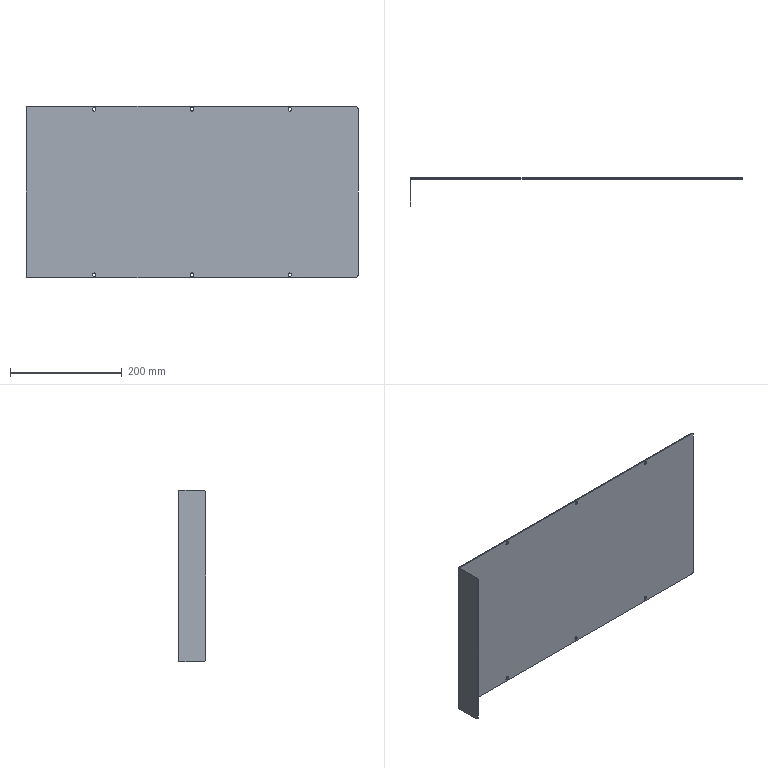Part | SolidWorks | features ICE 2, BreakCorner 1, EdgeFlange 1, Fillet 1, FlatPattern 1, SMBaseFlange 1, SheetMetal 1 | 1 solid | 48 faces | box 595 x 50 x 308 mm | volume 296830 mm3 | cylinder 24 | plane 24 | commonest cylinder face diameters 5 x18 10 x4 0.2 x1 3.2 x1
STEP:
#1=CARTESIAN_POINT('',(-175.,-1.5,-145.));
#2=VERTEX_POINT('',#1);
#3=CARTESIAN_POINT('',(-172.5,-1.5,-147.5));
#4=VERTEX_POINT('',#3);
#5=CARTESIAN_POINT('',(-175.,-1.5,-147.5));
#6=DIRECTION('',(0.,1.,0.));
#7=DIRECTION('',(0.,0.,1.));
#8=AXIS2_PLACEMENT_3D('',#5,#6,#7);
#9=CIRCLE('',#8,2.5);
#10=EDGE_CURVE('',#2,#4,#9,.T.);
#11=ORIENTED_EDGE('',*,*,#10,.F.);
#12=CARTESIAN_POINT('',(-175.,0.,-145.));
#13=VERTEX_POINT('',#12);
#14=CARTESIAN_POINT('',(-175.,-10.,-145.));
#15=DIRECTION('',(0.,1.,0.));
#16=VECTOR('',#15,1000.);
#17=LINE('',#14,#16);
#18=EDGE_CURVE('',#2,#13,#17,.T.);
#19=ORIENTED_EDGE('',*,*,#18,.T.);
#20=CARTESIAN_POINT('',(-172.5,0.,-147.5));
#21=VERTEX_POINT('',#20);
#22=CARTESIAN_POINT('',(-175.,0.,-147.5));
#23=DIRECTION('',(0.,1.,0.));
#24=DIRECTION('',(0.,0.,-1.));
#25=AXIS2_PLACEMENT_3D('',#22,#23,#24);
#26=CIRCLE('',#25,2.5);
#27=EDGE_CURVE('',#13,#21,#26,.T.);
#28=ORIENTED_EDGE('',*,*,#27,.T.);
#29=CARTESIAN_POINT('',(-172.5,-10.,-147.5));
#30=DIRECTION('',(0.,1.,0.));
#31=VECTOR('',#30,1000.);
#32=LINE('',#29,#31);
#33=EDGE_CURVE('',#4,#21,#32,.T.);
#34=ORIENTED_EDGE('',*,*,#33,.F.);
#35=EDGE_LOOP('',(#11,#19,#28,#34));
#36=FACE_OUTER_BOUND('',#35,.T.);
#37=CARTESIAN_POINT('',(-175.,-10.,-147.5));
#38=DIRECTION('',(0.,1.,0.));
#39=DIRECTION('',(0.,0.,1.));
#40=AXIS2_PLACEMENT_3D('',#37,#38,#39);
#41=CYLINDRICAL_SURFACE('',#40,2.5);
#42=ADVANCED_FACE('',(#36),#41,.F.);
#43=CARTESIAN_POINT('',(0.,-1.5,-145.));
#44=VERTEX_POINT('',#43);
#45=CARTESIAN_POINT('',(2.5,-1.5,-147.5));
#46=VERTEX_POINT('',#45);
#47=CARTESIAN_POINT('',(0.,-1.5,-147.5));
#48=DIRECTION('',(0.,1.,0.));
#49=DIRECTION('',(0.,0.,1.));
#50=AXIS2_PLACEMENT_3D('',#47,#48,#49);
#51=CIRCLE('',#50,2.5);
#52=EDGE_CURVE('',#44,#46,#51,.T.);
#53=ORIENTED_EDGE('',*,*,#52,.F.);
#54=CARTESIAN_POINT('',(0.,0.,-145.));
#55=VERTEX_POINT('',#54);
#56=CARTESIAN_POINT('',(0.,-10.,-145.));
#57=DIRECTION('',(0.,1.,0.));
#58=VECTOR('',#57,1000.);
#59=LINE('',#56,#58);
#60=EDGE_CURVE('',#44,#55,#59,.T.);
#61=ORIENTED_EDGE('',*,*,#60,.T.);
#62=CARTESIAN_POINT('',(2.5,0.,-147.5));
#63=VERTEX_POINT('',#62);
#64=CARTESIAN_POINT('',(0.,0.,-147.5));
#65=DIRECTION('',(0.,1.,0.));
#66=DIRECTION('',(0.,0.,-1.));
#67=AXIS2_PLACEMENT_3D('',#64,#65,#66);
#68=CIRCLE('',#67,2.5);
#69=EDGE_CURVE('',#55,#63,#68,.T.);
#70=ORIENTED_EDGE('',*,*,#69,.T.);
#71=CARTESIAN_POINT('',(2.5,-10.,-147.5));
#72=DIRECTION('',(0.,1.,0.));
#73=VECTOR('',#72,1000.);
#74=LINE('',#71,#73);
#75=EDGE_CURVE('',#46,#63,#74,.T.);
#76=ORIENTED_EDGE('',*,*,#75,.F.);
#77=EDGE_LOOP('',(#53,#61,#70,#76));
#78=FACE_OUTER_BOUND('',#77,.T.);
#79=CARTESIAN_POINT('',(0.,-10.,-147.5));
#80=DIRECTION('',(0.,1.,0.));
#81=DIRECTION('',(0.,0.,1.));
#82=AXIS2_PLACEMENT_3D('',#79,#80,#81);
#83=CYLINDRICAL_SURFACE('',#82,2.5);
#84=ADVANCED_FACE('',(#78),#83,.F.);
#85=CARTESIAN_POINT('',(175.,-1.5,-145.));
#86=VERTEX_POINT('',#85);
#87=CARTESIAN_POINT('',(177.5,-1.5,-147.5));
#88=VERTEX_POINT('',#87);
#89=CARTESIAN_POINT('',(175.,-1.5,-147.5));
#90=DIRECTION('',(0.,1.,0.));
#91=DIRECTION('',(0.,0.,1.));
#92=AXIS2_PLACEMENT_3D('',#89,#90,#91);
#93=CIRCLE('',#92,2.5);
#94=EDGE_CURVE('',#86,#88,#93,.T.);
#95=ORIENTED_EDGE('',*,*,#94,.F.);
#96=CARTESIAN_POINT('',(175.,0.,-145.));
#97=VERTEX_POINT('',#96);
#98=CARTESIAN_POINT('',(175.,-10.,-145.));
#99=DIRECTION('',(0.,1.,0.));
#100=VECTOR('',#99,1000.);
#101=LINE('',#98,#100);
#102=EDGE_CURVE('',#86,#97,#101,.T.);
#103=ORIENTED_EDGE('',*,*,#102,.T.);
#104=CARTESIAN_POINT('',(177.5,0.,-147.5));
#105=VERTEX_POINT('',#104);
#106=CARTESIAN_POINT('',(175.,0.,-147.5));
#107=DIRECTION('',(0.,1.,0.));
#108=DIRECTION('',(0.,0.,-1.));
#109=AXIS2_PLACEMENT_3D('',#106,#107,#108);
#110=CIRCLE('',#109,2.5);
#111=EDGE_CURVE('',#97,#105,#110,.T.);
#112=ORIENTED_EDGE('',*,*,#111,.T.);
#113=CARTESIAN_POINT('',(177.5,-10.,-147.5));
#114=DIRECTION('',(0.,1.,0.));
#115=VECTOR('',#114,1000.);
#116=LINE('',#113,#115);
#117=EDGE_CURVE('',#88,#105,#116,.T.);
#118=ORIENTED_EDGE('',*,*,#117,.F.);
#119=EDGE_LOOP('',(#95,#103,#112,#118));
#120=FACE_OUTER_BOUND('',#119,.T.);
#121=CARTESIAN_POINT('',(175.,-10.,-147.5));
#122=DIRECTION('',(0.,1.,0.));
#123=DIRECTION('',(0.,0.,1.));
#124=AXIS2_PLACEMENT_3D('',#121,#122,#123);
#125=CYLINDRICAL_SURFACE('',#124,2.5);
#126=ADVANCED_FACE('',(#120),#125,.F.);
#127=CARTESIAN_POINT('',(175.,-1.5,152.));
#128=VERTEX_POINT('',#127);
#129=CARTESIAN_POINT('',(177.5,-1.5,149.5));
#130=VERTEX_POINT('',#129);
#131=CARTESIAN_POINT('',(175.,-1.5,149.5));
#132=DIRECTION('',(0.,1.,0.));
#133=DIRECTION('',(0.,0.,1.));
#134=AXIS2_PLACEMENT_3D('',#131,#132,#133);
#135=CIRCLE('',#134,2.5);
#136=EDGE_CURVE('',#128,#130,#135,.T.);
#137=ORIENTED_EDGE('',*,*,#136,.F.);
#138=CARTESIAN_POINT('',(175.,0.,152.));
#139=VERTEX_POINT('',#138);
#140=CARTESIAN_POINT('',(175.,-10.,152.));
#141=DIRECTION('',(0.,1.,0.));
#142=VECTOR('',#141,1000.);
#143=LINE('',#140,#142);
#144=EDGE_CURVE('',#128,#139,#143,.T.);
#145=ORIENTED_EDGE('',*,*,#144,.T.);
#146=CARTESIAN_POINT('',(177.5,0.,149.5));
#147=VERTEX_POINT('',#146);
#148=CARTESIAN_POINT('',(175.,0.,149.5));
#149=DIRECTION('',(0.,1.,0.));
#150=DIRECTION('',(0.,0.,1.));
#151=AXIS2_PLACEMENT_3D('',#148,#149,#150);
#152=CIRCLE('',#151,2.5);
#153=EDGE_CURVE('',#139,#147,#152,.T.);
#154=ORIENTED_EDGE('',*,*,#153,.T.);
#155=CARTESIAN_POINT('',(177.5,-10.,149.5));
#156=DIRECTION('',(0.,1.,0.));
#157=VECTOR('',#156,1000.);
#158=LINE('',#155,#157);
#159=EDGE_CURVE('',#130,#147,#158,.T.);
#160=ORIENTED_EDGE('',*,*,#159,.F.);
#161=EDGE_LOOP('',(#137,#145,#154,#160));
#162=FACE_OUTER_BOUND('',#161,.T.);
#163=CARTESIAN_POINT('',(175.,-10.,149.5));
#164=DIRECTION('',(0.,1.,0.));
#165=DIRECTION('',(0.,0.,1.));
#166=AXIS2_PLACEMENT_3D('',#163,#164,#165);
#167=CYLINDRICAL_SURFACE('',#166,2.5);
#168=ADVANCED_FACE('',(#162),#167,.F.);
#169=CARTESIAN_POINT('',(0.,-1.5,152.));
#170=VERTEX_POINT('',#169);
#171=CARTESIAN_POINT('',(2.5,-1.5,149.5));
#172=VERTEX_POINT('',#171);
#173=CARTESIAN_POINT('',(0.,-1.5,149.5));
#174=DIRECTION('',(0.,1.,0.));
#175=DIRECTION('',(0.,0.,1.));
#176=AXIS2_PLACEMENT_3D('',#173,#174,#175);
#177=CIRCLE('',#176,2.5);
#178=EDGE_CURVE('',#170,#172,#177,.T.);
#179=ORIENTED_EDGE('',*,*,#178,.F.);
#180=CARTESIAN_POINT('',(0.,0.,152.));
#181=VERTEX_POINT('',#180);
#182=CARTESIAN_POINT('',(0.,-10.,152.));
#183=DIRECTION('',(0.,1.,0.));
#184=VECTOR('',#183,1000.);
#185=LINE('',#182,#184);
#186=EDGE_CURVE('',#170,#181,#185,.T.);
#187=ORIENTED_EDGE('',*,*,#186,.T.);
#188=CARTESIAN_POINT('',(2.5,0.,149.5));
#189=VERTEX_POINT('',#188);
#190=CARTESIAN_POINT('',(0.,0.,149.5));
#191=DIRECTION('',(0.,1.,0.));
#192=DIRECTION('',(0.,0.,1.));
#193=AXIS2_PLACEMENT_3D('',#190,#191,#192);
#194=CIRCLE('',#193,2.5);
#195=EDGE_CURVE('',#181,#189,#194,.T.);
#196=ORIENTED_EDGE('',*,*,#195,.T.);
#197=CARTESIAN_POINT('',(2.5,-10.,149.5));
#198=DIRECTION('',(0.,1.,0.));
#199=VECTOR('',#198,1000.);
#200=LINE('',#197,#199);
#201=EDGE_CURVE('',#172,#189,#200,.T.);
#202=ORIENTED_EDGE('',*,*,#201,.F.);
#203=EDGE_LOOP('',(#179,#187,#196,#202));
#204=FACE_OUTER_BOUND('',#203,.T.);
#205=CARTESIAN_POINT('',(0.,-10.,149.5));
#206=DIRECTION('',(0.,1.,0.));
#207=DIRECTION('',(0.,0.,1.));
#208=AXIS2_PLACEMENT_3D('',#205,#206,#207);
#209=CYLINDRICAL_SURFACE('',#208,2.5);
#210=ADVANCED_FACE('',(#204),#209,.F.);
#211=CARTESIAN_POINT('',(-175.,-1.5,152.));
#212=VERTEX_POINT('',#211);
#213=CARTESIAN_POINT('',(-172.5,-1.5,149.5));
#214=VERTEX_POINT('',#213);
#215=CARTESIAN_POINT('',(-175.,-1.5,149.5));
#216=DIRECTION('',(0.,1.,0.));
#217=DIRECTION('',(0.,0.,1.));
#218=AXIS2_PLACEMENT_3D('',#215,#216,#217);
#219=CIRCLE('',#218,2.5);
#220=EDGE_CURVE('',#212,#214,#219,.T.);
#221=ORIENTED_EDGE('',*,*,#220,.F.);
#222=CARTESIAN_POINT('',(-175.,0.,152.));
#223=VERTEX_POINT('',#222);
#224=CARTESIAN_POINT('',(-175.,-10.,152.));
#225=DIRECTION('',(0.,1.,0.));
#226=VECTOR('',#225,1000.);
#227=LINE('',#224,#226);
#228=EDGE_CURVE('',#212,#223,#227,.T.);
#229=ORIENTED_EDGE('',*,*,#228,.T.);
#230=CARTESIAN_POINT('',(-172.5,0.,149.5));
#231=VERTEX_POINT('',#230);
#232=CARTESIAN_POINT('',(-175.,0.,149.5));
#233=DIRECTION('',(0.,1.,0.));
#234=DIRECTION('',(0.,0.,1.));
#235=AXIS2_PLACEMENT_3D('',#232,#233,#234);
#236=CIRCLE('',#235,2.5);
#237=EDGE_CURVE('',#223,#231,#236,.T.);
#238=ORIENTED_EDGE('',*,*,#237,.T.);
#239=CARTESIAN_POINT('',(-172.5,-10.,149.5));
#240=DIRECTION('',(0.,1.,0.));
#241=VECTOR('',#240,1000.);
#242=LINE('',#239,#241);
#243=EDGE_CURVE('',#214,#231,#242,.T.);
#244=ORIENTED_EDGE('',*,*,#243,.F.);
#245=EDGE_LOOP('',(#221,#229,#238,#244));
#246=FACE_OUTER_BOUND('',#245,.T.);
#247=CARTESIAN_POINT('',(-175.,-10.,149.5));
#248=DIRECTION('',(0.,1.,0.));
#249=DIRECTION('',(0.,0.,1.));
#250=AXIS2_PLACEMENT_3D('',#247,#248,#249);
#251=CYLINDRICAL_SURFACE('',#250,2.5);
#252=ADVANCED_FACE('',(#246),#251,.F.);
#253=CARTESIAN_POINT('',(292.5,0.,-154.));
#254=VERTEX_POINT('',#253);
#255=CARTESIAN_POINT('',(-295.9,0.,-154.));
#256=VERTEX_POINT('',#255);
#257=CARTESIAN_POINT('',(297.5,0.,-154.));
#258=DIRECTION('',(-1.,0.,0.));
#259=VECTOR('',#258,1000.);
#260=LINE('',#257,#259);
#261=EDGE_CURVE('',#254,#256,#260,.T.);
#262=ORIENTED_EDGE('',*,*,#261,.F.);
#263=CARTESIAN_POINT('',(292.5,-1.5,-154.));
#264=VERTEX_POINT('',#263);
#265=CARTESIAN_POINT('',(292.5,-1.5,-154.));
#266=DIRECTION('',(0.,-1.,0.));
#267=VECTOR('',#266,1000.);
#268=LINE('',#265,#267);
#269=EDGE_CURVE('',#254,#264,#268,.T.);
#270=ORIENTED_EDGE('',*,*,#269,.T.);
#271=CARTESIAN_POINT('',(-295.9,-1.5,-154.));
#272=VERTEX_POINT('',#271);
#273=CARTESIAN_POINT('',(297.5,-1.5,-154.));
#274=DIRECTION('',(-1.,0.,0.));
#275=VECTOR('',#274,1000.);
#276=LINE('',#273,#275);
#277=EDGE_CURVE('',#264,#272,#276,.T.);
#278=ORIENTED_EDGE('',*,*,#277,.T.);
#279=CARTESIAN_POINT('',(-295.9,-1.5,-154.));
#280=DIRECTION('',(0.,1.,0.));
#281=VECTOR('',#280,1000.);
#282=LINE('',#279,#281);
#283=EDGE_CURVE('',#272,#256,#282,.T.);
#284=ORIENTED_EDGE('',*,*,#283,.T.);
#285=EDGE_LOOP('',(#262,#270,#278,#284));
#286=FACE_OUTER_BOUND('',#285,.T.);
#287=CARTESIAN_POINT('',(297.5,-1.5,-154.));
#288=DIRECTION('',(0.,0.,-1.));
#289=DIRECTION('',(-1.,0.,0.));
#290=AXIS2_PLACEMENT_3D('',#287,#288,#289);
#291=PLANE('',#290);
#292=ADVANCED_FACE('',(#286),#291,.T.);
#293=CARTESIAN_POINT('',(-172.5,-1.5,-149.5));
#294=VERTEX_POINT('',#293);
#295=CARTESIAN_POINT('',(-172.5,-1.5,0.));
#296=DIRECTION('',(0.,0.,-1.));
#297=VECTOR('',#296,1000.);
#298=LINE('',#295,#297);
#299=EDGE_CURVE('',#4,#294,#298,.T.);
#300=ORIENTED_EDGE('',*,*,#299,.T.);
#301=CARTESIAN_POINT('',(-177.5,-1.5,-149.5));
#302=VERTEX_POINT('',#301);
#303=CARTESIAN_POINT('',(-175.,-1.5,-149.5));
#304=DIRECTION('',(0.,1.,0.));
#305=DIRECTION('',(0.,0.,1.));
#306=AXIS2_PLACEMENT_3D('',#303,#304,#305);
#307=CIRCLE('',#306,2.5);
#308=EDGE_CURVE('',#294,#302,#307,.T.);
#309=ORIENTED_EDGE('',*,*,#308,.T.);
#310=CARTESIAN_POINT('',(-177.5,-1.5,-147.5));
#311=VERTEX_POINT('',#310);
#312=CARTESIAN_POINT('',(-177.5,-1.5,0.));
#313=DIRECTION('',(0.,0.,1.));
#314=VECTOR('',#313,1000.);
#315=LINE('',#312,#314);
#316=EDGE_CURVE('',#302,#311,#315,.T.);
#317=ORIENTED_EDGE('',*,*,#316,.T.);
#318=CARTESIAN_POINT('',(-175.,-1.5,-147.5));
#319=DIRECTION('',(0.,1.,0.));
#320=DIRECTION('',(0.,0.,1.));
#321=AXIS2_PLACEMENT_3D('',#318,#319,#320);
#322=CIRCLE('',#321,2.5);
#323=EDGE_CURVE('',#311,#2,#322,.T.);
#324=ORIENTED_EDGE('',*,*,#323,.T.);
#325=ORIENTED_EDGE('',*,*,#10,.T.);
#326=EDGE_LOOP('',(#300,#309,#317,#324,#325));
#327=FACE_BOUND('',#326,.T.);
#328=CARTESIAN_POINT('',(2.5,-1.5,-149.5));
#329=VERTEX_POINT('',#328);
#330=CARTESIAN_POINT('',(2.5,-1.5,0.));
#331=DIRECTION('',(0.,0.,-1.));
#332=VECTOR('',#331,1000.);
#333=LINE('',#330,#332);
#334=EDGE_CURVE('',#46,#329,#333,.T.);
#335=ORIENTED_EDGE('',*,*,#334,.T.);
#336=CARTESIAN_POINT('',(-2.5,-1.5,-149.5));
#337=VERTEX_POINT('',#336);
#338=CARTESIAN_POINT('',(0.,-1.5,-149.5));
#339=DIRECTION('',(0.,1.,0.));
#340=DIRECTION('',(0.,0.,1.));
#341=AXIS2_PLACEMENT_3D('',#338,#339,#340);
#342=CIRCLE('',#341,2.5);
#343=EDGE_CURVE('',#329,#337,#342,.T.);
#344=ORIENTED_EDGE('',*,*,#343,.T.);
#345=CARTESIAN_POINT('',(-2.5,-1.5,-147.5));
#346=VERTEX_POINT('',#345);
#347=CARTESIAN_POINT('',(-2.5,-1.5,0.));
#348=DIRECTION('',(0.,0.,1.));
#349=VECTOR('',#348,1000.);
#350=LINE('',#347,#349);
#351=EDGE_CURVE('',#337,#346,#350,.T.);
#352=ORIENTED_EDGE('',*,*,#351,.T.);
#353=CARTESIAN_POINT('',(0.,-1.5,-147.5));
#354=DIRECTION('',(0.,1.,0.));
#355=DIRECTION('',(0.,0.,1.));
#356=AXIS2_PLACEMENT_3D('',#353,#354,#355);
#357=CIRCLE('',#356,2.5);
#358=EDGE_CURVE('',#346,#44,#357,.T.);
#359=ORIENTED_EDGE('',*,*,#358,.T.);
#360=ORIENTED_EDGE('',*,*,#52,.T.);
#361=EDGE_LOOP('',(#335,#344,#352,#359,#360));
#362=FACE_BOUND('',#361,.T.);
#363=CARTESIAN_POINT('',(177.5,-1.5,-149.5));
#364=VERTEX_POINT('',#363);
#365=CARTESIAN_POINT('',(177.5,-1.5,0.));
#366=DIRECTION('',(0.,0.,-1.));
#367=VECTOR('',#366,1000.);
#368=LINE('',#365,#367);
#369=EDGE_CURVE('',#88,#364,#368,.T.);
#370=ORIENTED_EDGE('',*,*,#369,.T.);
#371=CARTESIAN_POINT('',(172.5,-1.5,-149.5));
#372=VERTEX_POINT('',#371);
#373=CARTESIAN_POINT('',(175.,-1.5,-149.5));
#374=DIRECTION('',(0.,1.,0.));
#375=DIRECTION('',(0.,0.,1.));
#376=AXIS2_PLACEMENT_3D('',#373,#374,#375);
#377=CIRCLE('',#376,2.5);
#378=EDGE_CURVE('',#364,#372,#377,.T.);
#379=ORIENTED_EDGE('',*,*,#378,.T.);
#380=CARTESIAN_POINT('',(172.5,-1.5,-147.5));
#381=VERTEX_POINT('',#380);
#382=CARTESIAN_POINT('',(172.5,-1.5,0.));
#383=DIRECTION('',(0.,0.,1.));
#384=VECTOR('',#383,1000.);
#385=LINE('',#382,#384);
#386=EDGE_CURVE('',#372,#381,#385,.T.);
#387=ORIENTED_EDGE('',*,*,#386,.T.);
#388=CARTESIAN_POINT('',(175.,-1.5,-147.5));
#389=DIRECTION('',(0.,1.,0.));
#390=DIRECTION('',(0.,0.,1.));
#391=AXIS2_PLACEMENT_3D('',#388,#389,#390);
#392=CIRCLE('',#391,2.5);
#393=EDGE_CURVE('',#381,#86,#392,.T.);
#394=ORIENTED_EDGE('',*,*,#393,.T.);
#395=ORIENTED_EDGE('',*,*,#94,.T.);
#396=EDGE_LOOP('',(#370,#379,#387,#394,#395));
#397=FACE_BOUND('',#396,.T.);
#398=CARTESIAN_POINT('',(172.5,-1.5,147.5));
#399=VERTEX_POINT('',#398);
#400=CARTESIAN_POINT('',(172.5,-1.5,149.5));
#401=VERTEX_POINT('',#400);
#402=CARTESIAN_POINT('',(172.5,-1.5,0.));
#403=DIRECTION('',(0.,0.,1.));
#404=VECTOR('',#403,1000.);
#405=LINE('',#402,#404);
#406=EDGE_CURVE('',#399,#401,#405,.T.);
#407=ORIENTED_EDGE('',*,*,#406,.T.);
#408=CARTESIAN_POINT('',(175.,-1.5,149.5));
#409=DIRECTION('',(0.,1.,0.));
#410=DIRECTION('',(0.,0.,1.));
#411=AXIS2_PLACEMENT_3D('',#408,#409,#410);
#412=CIRCLE('',#411,2.5);
#413=EDGE_CURVE('',#401,#128,#412,.T.);
#414=ORIENTED_EDGE('',*,*,#413,.T.);
#415=ORIENTED_EDGE('',*,*,#136,.T.);
#416=CARTESIAN_POINT('',(177.5,-1.5,147.5));
#417=VERTEX_POINT('',#416);
#418=CARTESIAN_POINT('',(177.5,-1.5,0.));
#419=DIRECTION('',(0.,0.,-1.));
#420=VECTOR('',#419,1000.);
#421=LINE('',#418,#420);
#422=EDGE_CURVE('',#130,#417,#421,.T.);
#423=ORIENTED_EDGE('',*,*,#422,.T.);
#424=CARTESIAN_POINT('',(175.,-1.5,147.5));
#425=DIRECTION('',(0.,1.,0.));
#426=DIRECTION('',(0.,0.,1.));
#427=AXIS2_PLACEMENT_3D('',#424,#425,#426);
#428=CIRCLE('',#427,2.5);
#429=EDGE_CURVE('',#417,#399,#428,.T.);
#430=ORIENTED_EDGE('',*,*,#429,.T.);
#431=EDGE_LOOP('',(#407,#414,#415,#423,#430));
#432=FACE_BOUND('',#431,.T.);
#433=CARTESIAN_POINT('',(-2.5,-1.5,147.5));
#434=VERTEX_POINT('',#433);
#435=CARTESIAN_POINT('',(-2.5,-1.5,149.5));
#436=VERTEX_POINT('',#435);
#437=CARTESIAN_POINT('',(-2.5,-1.5,0.));
#438=DIRECTION('',(0.,0.,1.));
#439=VECTOR('',#438,1000.);
#440=LINE('',#437,#439);
#441=EDGE_CURVE('',#434,#436,#440,.T.);
#442=ORIENTED_EDGE('',*,*,#441,.T.);
#443=CARTESIAN_POINT('',(0.,-1.5,149.5));
#444=DIRECTION('',(0.,1.,0.));
#445=DIRECTION('',(0.,0.,1.));
#446=AXIS2_PLACEMENT_3D('',#443,#444,#445);
#447=CIRCLE('',#446,2.5);
#448=EDGE_CURVE('',#436,#170,#447,.T.);
#449=ORIENTED_EDGE('',*,*,#448,.T.);
#450=ORIENTED_EDGE('',*,*,#178,.T.);
#451=CARTESIAN_POINT('',(2.5,-1.5,147.5));
#452=VERTEX_POINT('',#451);
#453=CARTESIAN_POINT('',(2.5,-1.5,0.));
#454=DIRECTION('',(0.,0.,-1.));
#455=VECTOR('',#454,1000.);
#456=LINE('',#453,#455);
#457=EDGE_CURVE('',#172,#452,#456,.T.);
#458=ORIENTED_EDGE('',*,*,#457,.T.);
#459=CARTESIAN_POINT('',(0.,-1.5,147.5));
#460=DIRECTION('',(0.,1.,0.));
#461=DIRECTION('',(0.,0.,1.));
#462=AXIS2_PLACEMENT_3D('',#459,#460,#461);
#463=CIRCLE('',#462,2.5);
#464=EDGE_CURVE('',#452,#434,#463,.T.);
#465=ORIENTED_EDGE('',*,*,#464,.T.);
#466=EDGE_LOOP('',(#442,#449,#450,#458,#465));
#467=FACE_BOUND('',#466,.T.);
#468=CARTESIAN_POINT('',(-177.5,-1.5,147.5));
#469=VERTEX_POINT('',#468);
#470=CARTESIAN_POINT('',(-177.5,-1.5,149.5));
#471=VERTEX_POINT('',#470);
#472=CARTESIAN_POINT('',(-177.5,-1.5,0.));
#473=DIRECTION('',(0.,0.,1.));
#474=VECTOR('',#473,1000.);
#475=LINE('',#472,#474);
#476=EDGE_CURVE('',#469,#471,#475,.T.);
#477=ORIENTED_EDGE('',*,*,#476,.T.);
#478=CARTESIAN_POINT('',(-175.,-1.5,149.5));
#479=DIRECTION('',(0.,1.,0.));
#480=DIRECTION('',(0.,0.,1.));
#481=AXIS2_PLACEMENT_3D('',#478,#479,#480);
#482=CIRCLE('',#481,2.5);
#483=EDGE_CURVE('',#471,#212,#482,.T.);
#484=ORIENTED_EDGE('',*,*,#483,.T.);
#485=ORIENTED_EDGE('',*,*,#220,.T.);
#486=CARTESIAN_POINT('',(-172.5,-1.5,147.5));
#487=VERTEX_POINT('',#486);
#488=CARTESIAN_POINT('',(-172.5,-1.5,0.));
#489=DIRECTION('',(0.,0.,-1.));
#490=VECTOR('',#489,1000.);
#491=LINE('',#488,#490);
#492=EDGE_CURVE('',#214,#487,#491,.T.);
#493=ORIENTED_EDGE('',*,*,#492,.T.);
#494=CARTESIAN_POINT('',(-175.,-1.5,147.5));
#495=DIRECTION('',(0.,1.,0.));
#496=DIRECTION('',(0.,0.,1.));
#497=AXIS2_PLACEMENT_3D('',#494,#495,#496);
#498=CIRCLE('',#497,2.5);
#499=EDGE_CURVE('',#487,#469,#498,.T.);
#500=ORIENTED_EDGE('',*,*,#499,.T.);
#501=EDGE_LOOP('',(#477,#484,#485,#493,#500));
#502=FACE_BOUND('',#501,.T.);
#503=CARTESIAN_POINT('',(297.5,-1.5,149.));
#504=VERTEX_POINT('',#503);
#505=CARTESIAN_POINT('',(297.5,-1.5,-149.));
#506=VERTEX_POINT('',#505);
#507=CARTESIAN_POINT('',(297.5,-1.5,154.));
#508=DIRECTION('',(0.,0.,-1.));
#509=VECTOR('',#508,1000.);
#510=LINE('',#507,#509);
#511=EDGE_CURVE('',#504,#506,#510,.T.);
#512=ORIENTED_EDGE('',*,*,#511,.F.);
#513=CARTESIAN_POINT('',(292.5,-1.5,154.));
#514=VERTEX_POINT('',#513);
#515=CARTESIAN_POINT('',(292.5,-1.5,149.));
#516=DIRECTION('',(0.,-1.,0.));
#517=DIRECTION('',(0.,0.,1.));
#518=AXIS2_PLACEMENT_3D('',#515,#516,#517);
#519=CIRCLE('',#518,5.);
#520=EDGE_CURVE('',#504,#514,#519,.T.);
#521=ORIENTED_EDGE('',*,*,#520,.T.);
#522=CARTESIAN_POINT('',(-295.9,-1.5,154.));
#523=VERTEX_POINT('',#522);
#524=CARTESIAN_POINT('',(297.5,-1.5,154.));
#525=DIRECTION('',(1.,0.,0.));
#526=VECTOR('',#525,1000.);
#527=LINE('',#524,#526);
#528=EDGE_CURVE('',#523,#514,#527,.T.);
#529=ORIENTED_EDGE('',*,*,#528,.F.);
#530=CARTESIAN_POINT('',(-295.9,-1.5,-154.));
#531=DIRECTION('',(0.,0.,1.));
#532=VECTOR('',#531,1000.);
#533=LINE('',#530,#532);
#534=EDGE_CURVE('',#272,#523,#533,.T.);
#535=ORIENTED_EDGE('',*,*,#534,.F.);
#536=ORIENTED_EDGE('',*,*,#277,.F.);
#537=CARTESIAN_POINT('',(292.5,-1.5,-149.));
#538=DIRECTION('',(0.,-1.,0.));
#539=DIRECTION('',(0.,0.,1.));
#540=AXIS2_PLACEMENT_3D('',#537,#538,#539);
#541=CIRCLE('',#540,5.);
#542=EDGE_CURVE('',#264,#506,#541,.T.);
#543=ORIENTED_EDGE('',*,*,#542,.T.);
#544=EDGE_LOOP('',(#512,#521,#529,#535,#536,#543));
#545=FACE_OUTER_BOUND('',#544,.T.);
#546=CARTESIAN_POINT('',(0.,-1.5,0.));
#547=DIRECTION('',(0.,1.,0.));
#548=DIRECTION('',(0.,0.,1.));
#549=AXIS2_PLACEMENT_3D('',#546,#547,#548);
#550=PLANE('',#549);
#551=ADVANCED_FACE('',(#327,#362,#397,#432,#467,#502,#545),#550,.F.);
#552=CARTESIAN_POINT('',(-172.5,0.,-149.5));
#553=VERTEX_POINT('',#552);
#554=CARTESIAN_POINT('',(-177.5,0.,-149.5));
#555=VERTEX_POINT('',#554);
#556=CARTESIAN_POINT('',(-175.,0.,-149.5));
#557=DIRECTION('',(0.,1.,0.));
#558=DIRECTION('',(0.,0.,-1.));
#559=AXIS2_PLACEMENT_3D('',#556,#557,#558);
#560=CIRCLE('',#559,2.5);
#561=EDGE_CURVE('',#553,#555,#560,.T.);
#562=ORIENTED_EDGE('',*,*,#561,.F.);
#563=CARTESIAN_POINT('',(-172.5,0.,-149.5));
#564=DIRECTION('',(0.,0.,-1.));
#565=VECTOR('',#564,1000.);
#566=LINE('',#563,#565);
#567=EDGE_CURVE('',#21,#553,#566,.T.);
#568=ORIENTED_EDGE('',*,*,#567,.F.);
#569=ORIENTED_EDGE('',*,*,#27,.F.);
#570=CARTESIAN_POINT('',(-177.5,0.,-147.5));
#571=VERTEX_POINT('',#570);
#572=CARTESIAN_POINT('',(-175.,0.,-147.5));
#573=DIRECTION('',(0.,1.,0.));
#574=DIRECTION('',(0.,0.,-1.));
#575=AXIS2_PLACEMENT_3D('',#572,#573,#574);
#576=CIRCLE('',#575,2.5);
#577=EDGE_CURVE('',#571,#13,#576,.T.);
#578=ORIENTED_EDGE('',*,*,#577,.F.);
#579=CARTESIAN_POINT('',(-177.5,0.,-149.5));
#580=DIRECTION('',(0.,0.,1.));
#581=VECTOR('',#580,1000.);
#582=LINE('',#579,#581);
#583=EDGE_CURVE('',#555,#571,#582,.T.);
#584=ORIENTED_EDGE('',*,*,#583,.F.);
#585=EDGE_LOOP('',(#562,#568,#569,#578,#584));
#586=FACE_BOUND('',#585,.T.);
#587=CARTESIAN_POINT('',(2.5,0.,-149.5));
#588=VERTEX_POINT('',#587);
#589=CARTESIAN_POINT('',(-2.5,0.,-149.5));
#590=VERTEX_POINT('',#589);
#591=CARTESIAN_POINT('',(0.,0.,-149.5));
#592=DIRECTION('',(0.,1.,0.));
#593=DIRECTION('',(0.,0.,-1.));
#594=AXIS2_PLACEMENT_3D('',#591,#592,#593);
#595=CIRCLE('',#594,2.5);
#596=EDGE_CURVE('',#588,#590,#595,.T.);
#597=ORIENTED_EDGE('',*,*,#596,.F.);
#598=CARTESIAN_POINT('',(2.5,0.,-149.5));
#599=DIRECTION('',(0.,0.,-1.));
#600=VECTOR('',#599,1000.);
#601=LINE('',#598,#600);
#602=EDGE_CURVE('',#63,#588,#601,.T.);
#603=ORIENTED_EDGE('',*,*,#602,.F.);
#604=ORIENTED_EDGE('',*,*,#69,.F.);
#605=CARTESIAN_POINT('',(-2.5,0.,-147.5));
#606=VERTEX_POINT('',#605);
#607=CARTESIAN_POINT('',(0.,0.,-147.5));
#608=DIRECTION('',(0.,1.,0.));
#609=DIRECTION('',(0.,0.,-1.));
#610=AXIS2_PLACEMENT_3D('',#607,#608,#609);
#611=CIRCLE('',#610,2.5);
#612=EDGE_CURVE('',#606,#55,#611,.T.);
#613=ORIENTED_EDGE('',*,*,#612,.F.);
#614=CARTESIAN_POINT('',(-2.5,0.,-149.5));
#615=DIRECTION('',(0.,0.,1.));
#616=VECTOR('',#615,1000.);
#617=LINE('',#614,#616);
#618=EDGE_CURVE('',#590,#606,#617,.T.);
#619=ORIENTED_EDGE('',*,*,#618,.F.);
#620=EDGE_LOOP('',(#597,#603,#604,#613,#619));
#621=FACE_BOUND('',#620,.T.);
#622=CARTESIAN_POINT('',(177.5,0.,-149.5));
#623=VERTEX_POINT('',#622);
#624=CARTESIAN_POINT('',(172.5,0.,-149.5));
#625=VERTEX_POINT('',#624);
#626=CARTESIAN_POINT('',(175.,0.,-149.5));
#627=DIRECTION('',(0.,1.,0.));
#628=DIRECTION('',(0.,0.,-1.));
#629=AXIS2_PLACEMENT_3D('',#626,#627,#628);
#630=CIRCLE('',#629,2.5);
#631=EDGE_CURVE('',#623,#625,#630,.T.);
#632=ORIENTED_EDGE('',*,*,#631,.F.);
#633=CARTESIAN_POINT('',(177.5,0.,-149.5));
#634=DIRECTION('',(0.,0.,-1.));
#635=VECTOR('',#634,1000.);
#636=LINE('',#633,#635);
#637=EDGE_CURVE('',#105,#623,#636,.T.);
#638=ORIENTED_EDGE('',*,*,#637,.F.);
#639=ORIENTED_EDGE('',*,*,#111,.F.);
#640=CARTESIAN_POINT('',(172.5,0.,-147.5));
#641=VERTEX_POINT('',#640);
#642=CARTESIAN_POINT('',(175.,0.,-147.5));
#643=DIRECTION('',(0.,1.,0.));
#644=DIRECTION('',(0.,0.,-1.));
#645=AXIS2_PLACEMENT_3D('',#642,#643,#644);
#646=CIRCLE('',#645,2.5);
#647=EDGE_CURVE('',#641,#97,#646,.T.);
#648=ORIENTED_EDGE('',*,*,#647,.F.);
#649=CARTESIAN_POINT('',(172.5,0.,-149.5));
#650=DIRECTION('',(0.,0.,1.));
#651=VECTOR('',#650,1000.);
#652=LINE('',#649,#651);
#653=EDGE_CURVE('',#625,#641,#652,.T.);
#654=ORIENTED_EDGE('',*,*,#653,.F.);
#655=EDGE_LOOP('',(#632,#638,#639,#648,#654));
#656=FACE_BOUND('',#655,.T.);
#657=CARTESIAN_POINT('',(172.5,0.,149.5));
#658=VERTEX_POINT('',#657);
#659=CARTESIAN_POINT('',(175.,0.,149.5));
#660=DIRECTION('',(0.,1.,0.));
#661=DIRECTION('',(0.,0.,1.));
#662=AXIS2_PLACEMENT_3D('',#659,#660,#661);
#663=CIRCLE('',#662,2.5);
#664=EDGE_CURVE('',#658,#139,#663,.T.);
#665=ORIENTED_EDGE('',*,*,#664,.F.);
#666=CARTESIAN_POINT('',(172.5,0.,147.5));
#667=VERTEX_POINT('',#666);
#668=CARTESIAN_POINT('',(172.5,0.,149.5));
#669=DIRECTION('',(0.,0.,1.));
#670=VECTOR('',#669,1000.);
#671=LINE('',#668,#670);
#672=EDGE_CURVE('',#667,#658,#671,.T.);
#673=ORIENTED_EDGE('',*,*,#672,.F.);
#674=CARTESIAN_POINT('',(177.5,0.,147.5));
#675=VERTEX_POINT('',#674);
#676=CARTESIAN_POINT('',(175.,0.,147.5));
#677=DIRECTION('',(0.,1.,0.));
#678=DIRECTION('',(0.,0.,1.));
#679=AXIS2_PLACEMENT_3D('',#676,#677,#678);
#680=CIRCLE('',#679,2.5);
#681=EDGE_CURVE('',#675,#667,#680,.T.);
#682=ORIENTED_EDGE('',*,*,#681,.F.);
#683=CARTESIAN_POINT('',(177.5,0.,149.5));
#684=DIRECTION('',(0.,0.,-1.));
#685=VECTOR('',#684,1000.);
#686=LINE('',#683,#685);
#687=EDGE_CURVE('',#147,#675,#686,.T.);
#688=ORIENTED_EDGE('',*,*,#687,.F.);
#689=ORIENTED_EDGE('',*,*,#153,.F.);
#690=EDGE_LOOP('',(#665,#673,#682,#688,#689));
#691=FACE_BOUND('',#690,.T.);
#692=CARTESIAN_POINT('',(-2.5,0.,149.5));
#693=VERTEX_POINT('',#692);
#694=CARTESIAN_POINT('',(0.,0.,149.5));
#695=DIRECTION('',(0.,1.,0.));
#696=DIRECTION('',(0.,0.,1.));
#697=AXIS2_PLACEMENT_3D('',#694,#695,#696);
#698=CIRCLE('',#697,2.5);
#699=EDGE_CURVE('',#693,#181,#698,.T.);
#700=ORIENTED_EDGE('',*,*,#699,.F.);
#701=CARTESIAN_POINT('',(-2.5,0.,147.5));
#702=VERTEX_POINT('',#701);
#703=CARTESIAN_POINT('',(-2.5,0.,149.5));
#704=DIRECTION('',(0.,0.,1.));
#705=VECTOR('',#704,1000.);
#706=LINE('',#703,#705);
#707=EDGE_CURVE('',#702,#693,#706,.T.);
#708=ORIENTED_EDGE('',*,*,#707,.F.);
#709=CARTESIAN_POINT('',(2.5,0.,147.5));
#710=VERTEX_POINT('',#709);
#711=CARTESIAN_POINT('',(0.,0.,147.5));
#712=DIRECTION('',(0.,1.,0.));
#713=DIRECTION('',(0.,0.,1.));
#714=AXIS2_PLACEMENT_3D('',#711,#712,#713);
#715=CIRCLE('',#714,2.5);
#716=EDGE_CURVE('',#710,#702,#715,.T.);
#717=ORIENTED_EDGE('',*,*,#716,.F.);
#718=CARTESIAN_POINT('',(2.5,0.,149.5));
#719=DIRECTION('',(0.,0.,-1.));
#720=VECTOR('',#719,1000.);
#721=LINE('',#718,#720);
#722=EDGE_CURVE('',#189,#710,#721,.T.);
#723=ORIENTED_EDGE('',*,*,#722,.F.);
#724=ORIENTED_EDGE('',*,*,#195,.F.);
#725=EDGE_LOOP('',(#700,#708,#717,#723,#724));
#726=FACE_BOUND('',#725,.T.);
#727=CARTESIAN_POINT('',(-177.5,0.,149.5));
#728=VERTEX_POINT('',#727);
#729=CARTESIAN_POINT('',(-175.,0.,149.5));
#730=DIRECTION('',(0.,1.,0.));
#731=DIRECTION('',(0.,0.,1.));
#732=AXIS2_PLACEMENT_3D('',#729,#730,#731);
#733=CIRCLE('',#732,2.5);
#734=EDGE_CURVE('',#728,#223,#733,.T.);
#735=ORIENTED_EDGE('',*,*,#734,.F.);
#736=CARTESIAN_POINT('',(-177.5,0.,147.5));
#737=VERTEX_POINT('',#736);
#738=CARTESIAN_POINT('',(-177.5,0.,149.5));
#739=DIRECTION('',(0.,0.,1.));
#740=VECTOR('',#739,1000.);
#741=LINE('',#738,#740);
#742=EDGE_CURVE('',#737,#728,#741,.T.);
#743=ORIENTED_EDGE('',*,*,#742,.F.);
#744=CARTESIAN_POINT('',(-172.5,0.,147.5));
#745=VERTEX_POINT('',#744);
#746=CARTESIAN_POINT('',(-175.,0.,147.5));
#747=DIRECTION('',(0.,1.,0.));
#748=DIRECTION('',(0.,0.,1.));
#749=AXIS2_PLACEMENT_3D('',#746,#747,#748);
#750=CIRCLE('',#749,2.5);
#751=EDGE_CURVE('',#745,#737,#750,.T.);
#752=ORIENTED_EDGE('',*,*,#751,.F.);
#753=CARTESIAN_POINT('',(-172.5,0.,149.5));
#754=DIRECTION('',(0.,0.,-1.));
#755=VECTOR('',#754,1000.);
#756=LINE('',#753,#755);
#757=EDGE_CURVE('',#231,#745,#756,.T.);
#758=ORIENTED_EDGE('',*,*,#757,.F.);
#759=ORIENTED_EDGE('',*,*,#237,.F.);
#760=EDGE_LOOP('',(#735,#743,#752,#758,#759));
#761=FACE_BOUND('',#760,.T.);
#762=CARTESIAN_POINT('',(-295.9,0.,154.));
#763=VERTEX_POINT('',#762);
#764=CARTESIAN_POINT('',(292.5,0.,154.));
#765=VERTEX_POINT('',#764);
#766=CARTESIAN_POINT('',(297.5,0.,154.));
#767=DIRECTION('',(1.,0.,0.));
#768=VECTOR('',#767,1000.);
#769=LINE('',#766,#768);
#770=EDGE_CURVE('',#763,#765,#769,.T.);
#771=ORIENTED_EDGE('',*,*,#770,.T.);
#772=CARTESIAN_POINT('',(297.5,0.,149.));
#773=VERTEX_POINT('',#772);
#774=CARTESIAN_POINT('',(292.5,0.,149.));
#775=DIRECTION('',(0.,1.,0.));
#776=DIRECTION('',(0.,0.,1.));
#777=AXIS2_PLACEMENT_3D('',#774,#775,#776);
#778=CIRCLE('',#777,5.);
#779=EDGE_CURVE('',#765,#773,#778,.T.);
#780=ORIENTED_EDGE('',*,*,#779,.T.);
#781=CARTESIAN_POINT('',(297.5,0.,-149.));
#782=VERTEX_POINT('',#781);
#783=CARTESIAN_POINT('',(297.5,0.,154.));
#784=DIRECTION('',(0.,0.,-1.));
#785=VECTOR('',#784,1000.);
#786=LINE('',#783,#785);
#787=EDGE_CURVE('',#773,#782,#786,.T.);
#788=ORIENTED_EDGE('',*,*,#787,.T.);
#789=CARTESIAN_POINT('',(292.5,0.,-149.));
#790=DIRECTION('',(0.,1.,0.));
#791=DIRECTION('',(0.,0.,1.));
#792=AXIS2_PLACEMENT_3D('',#789,#790,#791);
#793=CIRCLE('',#792,5.);
#794=EDGE_CURVE('',#782,#254,#793,.T.);
#795=ORIENTED_EDGE('',*,*,#794,.T.);
#796=ORIENTED_EDGE('',*,*,#261,.T.);
#797=CARTESIAN_POINT('',(-295.9,0.,-154.));
#798=DIRECTION('',(0.,0.,1.));
#799=VECTOR('',#798,1000.);
#800=LINE('',#797,#799);
#801=EDGE_CURVE('',#256,#763,#800,.T.);
#802=ORIENTED_EDGE('',*,*,#801,.T.);
#803=EDGE_LOOP('',(#771,#780,#788,#795,#796,#802));
#804=FACE_OUTER_BOUND('',#803,.T.);
#805=CARTESIAN_POINT('',(0.,0.,0.));
#806=DIRECTION('',(0.,1.,0.));
#807=DIRECTION('',(0.,0.,1.));
#808=AXIS2_PLACEMENT_3D('',#805,#806,#807);
#809=PLANE('',#808);
#810=ADVANCED_FACE('',(#586,#621,#656,#691,#726,#761,#804),#809,.T.);
#811=ORIENTED_EDGE('',*,*,#787,.F.);
#812=CARTESIAN_POINT('',(297.5,-1.5,149.));
#813=DIRECTION('',(0.,-1.,0.));
#814=VECTOR('',#813,1000.);
#815=LINE('',#812,#814);
#816=EDGE_CURVE('',#773,#504,#815,.T.);
#817=ORIENTED_EDGE('',*,*,#816,.T.);
#818=ORIENTED_EDGE('',*,*,#511,.T.);
#819=CARTESIAN_POINT('',(297.5,-1.5,-149.));
#820=DIRECTION('',(0.,1.,0.));
#821=VECTOR('',#820,1000.);
#822=LINE('',#819,#821);
#823=EDGE_CURVE('',#506,#782,#822,.T.);
#824=ORIENTED_EDGE('',*,*,#823,.T.);
#825=EDGE_LOOP('',(#811,#817,#818,#824));
#826=FACE_OUTER_BOUND('',#825,.T.);
#827=CARTESIAN_POINT('',(297.5,-1.5,154.));
#828=DIRECTION('',(1.,0.,0.));
#829=DIRECTION('',(0.,0.,-1.));
#830=AXIS2_PLACEMENT_3D('',#827,#828,#829);
#831=PLANE('',#830);
#832=ADVANCED_FACE('',(#826),#831,.T.);
#833=ORIENTED_EDGE('',*,*,#528,.T.);
#834=CARTESIAN_POINT('',(292.5,-1.5,154.));
#835=DIRECTION('',(0.,1.,0.));
#836=VECTOR('',#835,1000.);
#837=LINE('',#834,#836);
#838=EDGE_CURVE('',#514,#765,#837,.T.);
#839=ORIENTED_EDGE('',*,*,#838,.T.);
#840=ORIENTED_EDGE('',*,*,#770,.F.);
#841=CARTESIAN_POINT('',(-295.9,-1.5,154.));
#842=DIRECTION('',(0.,1.,0.));
#843=VECTOR('',#842,1000.);
#844=LINE('',#841,#843);
#845=EDGE_CURVE('',#523,#763,#844,.T.);
#846=ORIENTED_EDGE('',*,*,#845,.F.);
#847=EDGE_LOOP('',(#833,#839,#840,#846));
#848=FACE_OUTER_BOUND('',#847,.T.);
#849=CARTESIAN_POINT('',(297.5,-1.5,154.));
#850=DIRECTION('',(0.,0.,1.));
#851=DIRECTION('',(1.,0.,0.));
#852=AXIS2_PLACEMENT_3D('',#849,#850,#851);
#853=PLANE('',#852);
#854=ADVANCED_FACE('',(#848),#853,.T.);
#855=CARTESIAN_POINT('',(-296.,-1.6,154.));
#856=VERTEX_POINT('',#855);
#857=CARTESIAN_POINT('',(-297.5,-1.6,154.));
#858=VERTEX_POINT('',#857);
#859=CARTESIAN_POINT('',(-297.5,-1.6,154.));
#860=DIRECTION('',(-1.,0.,0.));
#861=VECTOR('',#860,1000.);
#862=LINE('',#859,#861);
#863=EDGE_CURVE('',#856,#858,#862,.T.);
#864=ORIENTED_EDGE('',*,*,#863,.F.);
#865=CARTESIAN_POINT('',(-295.9,-1.6,154.));
#866=DIRECTION('',(0.,0.,1.));
#867=DIRECTION('',(-1.,0.,0.));
#868=AXIS2_PLACEMENT_3D('',#865,#866,#867);
#869=CIRCLE('',#868,0.1);
#870=EDGE_CURVE('',#523,#856,#869,.T.);
#871=ORIENTED_EDGE('',*,*,#870,.F.);
#872=ORIENTED_EDGE('',*,*,#845,.T.);
#873=CARTESIAN_POINT('',(-295.9,-1.6,154.));
#874=DIRECTION('',(0.,0.,1.));
#875=DIRECTION('',(-1.,0.,0.));
#876=AXIS2_PLACEMENT_3D('',#873,#874,#875);
#877=CIRCLE('',#876,1.6);
#878=EDGE_CURVE('',#763,#858,#877,.T.);
#879=ORIENTED_EDGE('',*,*,#878,.T.);
#880=EDGE_LOOP('',(#864,#871,#872,#879));
#881=FACE_OUTER_BOUND('',#880,.T.);
#882=CARTESIAN_POINT('',(-295.9,-1.6,154.));
#883=DIRECTION('',(0.,0.,1.));
#884=DIRECTION('',(1.,0.,0.));
#885=AXIS2_PLACEMENT_3D('',#882,#883,#884);
#886=PLANE('',#885);
#887=ADVANCED_FACE('',(#881),#886,.T.);
#888=CARTESIAN_POINT('',(-296.,-1.6,-154.));
#889=VERTEX_POINT('',#888);
#890=CARTESIAN_POINT('',(-295.9,-1.6,-154.));
#891=DIRECTION('',(0.,0.,-1.));
#892=DIRECTION('',(-1.,0.,0.));
#893=AXIS2_PLACEMENT_3D('',#890,#891,#892);
#894=CIRCLE('',#893,0.1);
#895=EDGE_CURVE('',#889,#272,#894,.T.);
#896=ORIENTED_EDGE('',*,*,#895,.F.);
#897=CARTESIAN_POINT('',(-297.5,-1.6,-154.));
#898=VERTEX_POINT('',#897);
#899=CARTESIAN_POINT('',(-296.,-1.6,-154.));
#900=DIRECTION('',(-1.,0.,0.));
#901=VECTOR('',#900,1000.);
#902=LINE('',#899,#901);
#903=EDGE_CURVE('',#889,#898,#902,.T.);
#904=ORIENTED_EDGE('',*,*,#903,.T.);
#905=CARTESIAN_POINT('',(-295.9,-1.6,-154.));
#906=DIRECTION('',(0.,0.,-1.));
#907=DIRECTION('',(-1.,0.,0.));
#908=AXIS2_PLACEMENT_3D('',#905,#906,#907);
#909=CIRCLE('',#908,1.6);
#910=EDGE_CURVE('',#898,#256,#909,.T.);
#911=ORIENTED_EDGE('',*,*,#910,.T.);
#912=ORIENTED_EDGE('',*,*,#283,.F.);
#913=EDGE_LOOP('',(#896,#904,#911,#912));
#914=FACE_OUTER_BOUND('',#913,.T.);
#915=CARTESIAN_POINT('',(-295.9,-1.6,-154.));
#916=DIRECTION('',(0.,0.,1.));
#917=DIRECTION('',(1.,0.,0.));
#918=AXIS2_PLACEMENT_3D('',#915,#916,#917);
#919=PLANE('',#918);
#920=ADVANCED_FACE('',(#914),#919,.F.);
#921=ORIENTED_EDGE('',*,*,#801,.F.);
#922=ORIENTED_EDGE('',*,*,#910,.F.);
#923=CARTESIAN_POINT('',(-297.5,-1.6,0.));
#924=DIRECTION('',(0.,0.,-1.));
#925=VECTOR('',#924,1000.);
#926=LINE('',#923,#925);
#927=EDGE_CURVE('',#858,#898,#926,.T.);
#928=ORIENTED_EDGE('',*,*,#927,.F.);
#929=ORIENTED_EDGE('',*,*,#878,.F.);
#930=EDGE_LOOP('',(#921,#922,#928,#929));
#931=FACE_OUTER_BOUND('',#930,.T.);
#932=CARTESIAN_POINT('',(-295.9,-1.6,-154.));
#933=DIRECTION('',(0.,0.,-1.));
#934=DIRECTION('',(-1.,0.,0.));
#935=AXIS2_PLACEMENT_3D('',#932,#933,#934);
#936=CYLINDRICAL_SURFACE('',#935,1.6);
#937=ADVANCED_FACE('',(#931),#936,.T.);
#938=ORIENTED_EDGE('',*,*,#534,.T.);
#939=ORIENTED_EDGE('',*,*,#870,.T.);
#940=CARTESIAN_POINT('',(-296.,-1.6,154.));
#941=DIRECTION('',(0.,0.,-1.));
#942=VECTOR('',#941,1000.);
#943=LINE('',#940,#942);
#944=EDGE_CURVE('',#856,#889,#943,.T.);
#945=ORIENTED_EDGE('',*,*,#944,.T.);
#946=ORIENTED_EDGE('',*,*,#895,.T.);
#947=EDGE_LOOP('',(#938,#939,#945,#946));
#948=FACE_OUTER_BOUND('',#947,.T.);
#949=CARTESIAN_POINT('',(-295.9,-1.6,-154.));
#950=DIRECTION('',(0.,0.,-1.));
#951=DIRECTION('',(-1.,0.,0.));
#952=AXIS2_PLACEMENT_3D('',#949,#950,#951);
#953=CYLINDRICAL_SURFACE('',#952,0.1);
#954=ADVANCED_FACE('',(#948),#953,.F.);
#955=CARTESIAN_POINT('',(-296.,-45.,-154.));
#956=VERTEX_POINT('',#955);
#957=CARTESIAN_POINT('',(-296.,0.,-154.));
#958=DIRECTION('',(0.,1.,0.));
#959=VECTOR('',#958,1000.);
#960=LINE('',#957,#959);
#961=EDGE_CURVE('',#956,#889,#960,.T.);
#962=ORIENTED_EDGE('',*,*,#961,.F.);
#963=CARTESIAN_POINT('',(-297.5,-45.,-154.));
#964=VERTEX_POINT('',#963);
#965=CARTESIAN_POINT('',(-297.5,-45.,-154.));
#966=DIRECTION('',(-1.,0.,0.));
#967=VECTOR('',#966,1000.);
#968=LINE('',#965,#967);
#969=EDGE_CURVE('',#956,#964,#968,.T.);
#970=ORIENTED_EDGE('',*,*,#969,.T.);
#971=CARTESIAN_POINT('',(-297.5,-1.5,-154.));
#972=DIRECTION('',(0.,1.,0.));
#973=VECTOR('',#972,1000.);
#974=LINE('',#971,#973);
#975=EDGE_CURVE('',#964,#898,#974,.T.);
#976=ORIENTED_EDGE('',*,*,#975,.T.);
#977=ORIENTED_EDGE('',*,*,#903,.F.);
#978=EDGE_LOOP('',(#962,#970,#976,#977));
#979=FACE_OUTER_BOUND('',#978,.T.);
#980=CARTESIAN_POINT('',(-297.5,-1.5,-154.));
#981=DIRECTION('',(0.,0.,-1.));
#982=DIRECTION('',(0.,1.,0.));
#983=AXIS2_PLACEMENT_3D('',#980,#981,#982);
#984=PLANE('',#983);
#985=ADVANCED_FACE('',(#979),#984,.T.);
#986=CARTESIAN_POINT('',(-297.5,-45.,154.));
#987=VERTEX_POINT('',#986);
#988=CARTESIAN_POINT('',(-297.5,-50.,154.));
#989=DIRECTION('',(0.,-1.,0.));
#990=VECTOR('',#989,1000.);
#991=LINE('',#988,#990);
#992=EDGE_CURVE('',#858,#987,#991,.T.);
#993=ORIENTED_EDGE('',*,*,#992,.T.);
#994=CARTESIAN_POINT('',(-296.,-45.,154.));
#995=VERTEX_POINT('',#994);
#996=CARTESIAN_POINT('',(-297.5,-45.,154.));
#997=DIRECTION('',(1.,0.,0.));
#998=VECTOR('',#997,1000.);
#999=LINE('',#996,#998);
#1000=EDGE_CURVE('',#987,#995,#999,.T.);
#1001=ORIENTED_EDGE('',*,*,#1000,.T.);
#1002=CARTESIAN_POINT('',(-296.,0.,154.));
#1003=DIRECTION('',(0.,-1.,0.));
#1004=VECTOR('',#1003,1000.);
#1005=LINE('',#1002,#1004);
#1006=EDGE_CURVE('',#856,#995,#1005,.T.);
#1007=ORIENTED_EDGE('',*,*,#1006,.F.);
#1008=ORIENTED_EDGE('',*,*,#863,.T.);
#1009=EDGE_LOOP('',(#993,#1001,#1007,#1008));
#1010=FACE_OUTER_BOUND('',#1009,.T.);
#1011=CARTESIAN_POINT('',(-297.5,-50.,154.));
#1012=DIRECTION('',(0.,0.,1.));
#1013=DIRECTION('',(0.,-1.,0.));
#1014=AXIS2_PLACEMENT_3D('',#1011,#1012,#1013);
#1015=PLANE('',#1014);
#1016=ADVANCED_FACE('',(#1010),#1015,.T.);
#1017=ORIENTED_EDGE('',*,*,#975,.F.);
#1018=CARTESIAN_POINT('',(-297.5,-50.,-149.));
#1019=VERTEX_POINT('',#1018);
#1020=CARTESIAN_POINT('',(-297.5,-45.,-149.));
#1021=DIRECTION('',(-1.,0.,0.));
#1022=DIRECTION('',(0.,-1.,0.));
#1023=AXIS2_PLACEMENT_3D('',#1020,#1021,#1022);
#1024=CIRCLE('',#1023,5.);
#1025=EDGE_CURVE('',#964,#1019,#1024,.T.);
#1026=ORIENTED_EDGE('',*,*,#1025,.T.);
#1027=CARTESIAN_POINT('',(-297.5,-50.,149.));
#1028=VERTEX_POINT('',#1027);
#1029=CARTESIAN_POINT('',(-297.5,-50.,-154.));
#1030=DIRECTION('',(0.,0.,-1.));
#1031=VECTOR('',#1030,1000.);
#1032=LINE('',#1029,#1031);
#1033=EDGE_CURVE('',#1028,#1019,#1032,.T.);
#1034=ORIENTED_EDGE('',*,*,#1033,.F.);
#1035=CARTESIAN_POINT('',(-297.5,-45.,149.));
#1036=DIRECTION('',(-1.,0.,0.));
#1037=DIRECTION('',(0.,-1.,0.));
#1038=AXIS2_PLACEMENT_3D('',#1035,#1036,#1037);
#1039=CIRCLE('',#1038,5.);
#1040=EDGE_CURVE('',#1028,#987,#1039,.T.);
#1041=ORIENTED_EDGE('',*,*,#1040,.T.);
#1042=ORIENTED_EDGE('',*,*,#992,.F.);
#1043=ORIENTED_EDGE('',*,*,#927,.T.);
#1044=EDGE_LOOP('',(#1017,#1026,#1034,#1041,#1042,#1043));
#1045=FACE_OUTER_BOUND('',#1044,.T.);
#1046=CARTESIAN_POINT('',(-297.5,0.,0.));
#1047=DIRECTION('',(-1.,0.,0.));
#1048=DIRECTION('',(0.,-1.,0.));
#1049=AXIS2_PLACEMENT_3D('',#1046,#1047,#1048);
#1050=PLANE('',#1049);
#1051=ADVANCED_FACE('',(#1045),#1050,.T.);
#1052=CARTESIAN_POINT('',(-296.,-50.,149.));
#1053=VERTEX_POINT('',#1052);
#1054=CARTESIAN_POINT('',(-296.,-50.,-149.));
#1055=VERTEX_POINT('',#1054);
#1056=CARTESIAN_POINT('',(-296.,-50.,0.));
#1057=DIRECTION('',(0.,0.,-1.));
#1058=VECTOR('',#1057,1000.);
#1059=LINE('',#1056,#1058);
#1060=EDGE_CURVE('',#1053,#1055,#1059,.T.);
#1061=ORIENTED_EDGE('',*,*,#1060,.T.);
#1062=CARTESIAN_POINT('',(-296.,-45.,-149.));
#1063=DIRECTION('',(1.,0.,0.));
#1064=DIRECTION('',(0.,-1.,0.));
#1065=AXIS2_PLACEMENT_3D('',#1062,#1063,#1064);
#1066=CIRCLE('',#1065,5.);
#1067=EDGE_CURVE('',#1055,#956,#1066,.T.);
#1068=ORIENTED_EDGE('',*,*,#1067,.T.);
#1069=ORIENTED_EDGE('',*,*,#961,.T.);
#1070=ORIENTED_EDGE('',*,*,#944,.F.);
#1071=ORIENTED_EDGE('',*,*,#1006,.T.);
#1072=CARTESIAN_POINT('',(-296.,-45.,149.));
#1073=DIRECTION('',(1.,0.,0.));
#1074=DIRECTION('',(0.,-1.,0.));
#1075=AXIS2_PLACEMENT_3D('',#1072,#1073,#1074);
#1076=CIRCLE('',#1075,5.);
#1077=EDGE_CURVE('',#995,#1053,#1076,.T.);
#1078=ORIENTED_EDGE('',*,*,#1077,.T.);
#1079=EDGE_LOOP('',(#1061,#1068,#1069,#1070,#1071,#1078));
#1080=FACE_OUTER_BOUND('',#1079,.T.);
#1081=CARTESIAN_POINT('',(-296.,0.,0.));
#1082=DIRECTION('',(-1.,0.,0.));
#1083=DIRECTION('',(0.,-1.,0.));
#1084=AXIS2_PLACEMENT_3D('',#1081,#1082,#1083);
#1085=PLANE('',#1084);
#1086=ADVANCED_FACE('',(#1080),#1085,.F.);
#1087=ORIENTED_EDGE('',*,*,#1033,.T.);
#1088=CARTESIAN_POINT('',(-297.5,-50.,-149.));
#1089=DIRECTION('',(1.,0.,0.));
#1090=VECTOR('',#1089,1000.);
#1091=LINE('',#1088,#1090);
#1092=EDGE_CURVE('',#1019,#1055,#1091,.T.);
#1093=ORIENTED_EDGE('',*,*,#1092,.T.);
#1094=ORIENTED_EDGE('',*,*,#1060,.F.);
#1095=CARTESIAN_POINT('',(-297.5,-50.,149.));
#1096=DIRECTION('',(-1.,0.,0.));
#1097=VECTOR('',#1096,1000.);
#1098=LINE('',#1095,#1097);
#1099=EDGE_CURVE('',#1053,#1028,#1098,.T.);
#1100=ORIENTED_EDGE('',*,*,#1099,.T.);
#1101=EDGE_LOOP('',(#1087,#1093,#1094,#1100));
#1102=FACE_OUTER_BOUND('',#1101,.T.);
#1103=CARTESIAN_POINT('',(-297.5,-50.,-154.));
#1104=DIRECTION('',(0.,-1.,0.));
#1105=DIRECTION('',(1.,0.,0.));
#1106=AXIS2_PLACEMENT_3D('',#1103,#1104,#1105);
#1107=PLANE('',#1106);
#1108=ADVANCED_FACE('',(#1102),#1107,.T.);
#1109=ORIENTED_EDGE('',*,*,#228,.F.);
#1110=ORIENTED_EDGE('',*,*,#483,.F.);
#1111=CARTESIAN_POINT('',(-177.5,-10.,149.5));
#1112=DIRECTION('',(0.,1.,0.));
#1113=VECTOR('',#1112,1000.);
#1114=LINE('',#1111,#1113);
#1115=EDGE_CURVE('',#471,#728,#1114,.T.);
#1116=ORIENTED_EDGE('',*,*,#1115,.T.);
#1117=ORIENTED_EDGE('',*,*,#734,.T.);
#1118=EDGE_LOOP('',(#1109,#1110,#1116,#1117));
#1119=FACE_OUTER_BOUND('',#1118,.T.);
#1120=CARTESIAN_POINT('',(-175.,-10.,149.5));
#1121=DIRECTION('',(0.,1.,0.));
#1122=DIRECTION('',(0.,0.,1.));
#1123=AXIS2_PLACEMENT_3D('',#1120,#1121,#1122);
#1124=CYLINDRICAL_SURFACE('',#1123,2.5);
#1125=ADVANCED_FACE('',(#1119),#1124,.F.);
#1126=CARTESIAN_POINT('',(-177.5,-10.,147.5));
#1127=DIRECTION('',(0.,1.,0.));
#1128=VECTOR('',#1127,1000.);
#1129=LINE('',#1126,#1128);
#1130=EDGE_CURVE('',#469,#737,#1129,.T.);
#1131=ORIENTED_EDGE('',*,*,#1130,.T.);
#1132=ORIENTED_EDGE('',*,*,#742,.T.);
#1133=ORIENTED_EDGE('',*,*,#1115,.F.);
#1134=ORIENTED_EDGE('',*,*,#476,.F.);
#1135=EDGE_LOOP('',(#1131,#1132,#1133,#1134));
#1136=FACE_OUTER_BOUND('',#1135,.T.);
#1137=CARTESIAN_POINT('',(-177.5,-10.,149.5));
#1138=DIRECTION('',(-1.,0.,0.));
#1139=DIRECTION('',(0.,0.,1.));
#1140=AXIS2_PLACEMENT_3D('',#1137,#1138,#1139);
#1141=PLANE('',#1140);
#1142=ADVANCED_FACE('',(#1136),#1141,.F.);
#1143=CARTESIAN_POINT('',(-172.5,-10.,147.5));
#1144=DIRECTION('',(0.,1.,0.));
#1145=VECTOR('',#1144,1000.);
#1146=LINE('',#1143,#1145);
#1147=EDGE_CURVE('',#487,#745,#1146,.T.);
#1148=ORIENTED_EDGE('',*,*,#1147,.T.);
#1149=ORIENTED_EDGE('',*,*,#751,.T.);
#1150=ORIENTED_EDGE('',*,*,#1130,.F.);
#1151=ORIENTED_EDGE('',*,*,#499,.F.);
#1152=EDGE_LOOP('',(#1148,#1149,#1150,#1151));
#1153=FACE_OUTER_BOUND('',#1152,.T.);
#1154=CARTESIAN_POINT('',(-175.,-10.,147.5));
#1155=DIRECTION('',(0.,1.,0.));
#1156=DIRECTION('',(0.,0.,1.));
#1157=AXIS2_PLACEMENT_3D('',#1154,#1155,#1156);
#1158=CYLINDRICAL_SURFACE('',#1157,2.5);
#1159=ADVANCED_FACE('',(#1153),#1158,.F.);
#1160=ORIENTED_EDGE('',*,*,#243,.T.);
#1161=ORIENTED_EDGE('',*,*,#757,.T.);
#1162=ORIENTED_EDGE('',*,*,#1147,.F.);
#1163=ORIENTED_EDGE('',*,*,#492,.F.);
#1164=EDGE_LOOP('',(#1160,#1161,#1162,#1163));
#1165=FACE_OUTER_BOUND('',#1164,.T.);
#1166=CARTESIAN_POINT('',(-172.5,-10.,149.5));
#1167=DIRECTION('',(1.,0.,0.));
#1168=DIRECTION('',(0.,0.,-1.));
#1169=AXIS2_PLACEMENT_3D('',#1166,#1167,#1168);
#1170=PLANE('',#1169);
#1171=ADVANCED_FACE('',(#1165),#1170,.F.);
#1172=ORIENTED_EDGE('',*,*,#186,.F.);
#1173=ORIENTED_EDGE('',*,*,#448,.F.);
#1174=CARTESIAN_POINT('',(-2.5,-10.,149.5));
#1175=DIRECTION('',(0.,1.,0.));
#1176=VECTOR('',#1175,1000.);
#1177=LINE('',#1174,#1176);
#1178=EDGE_CURVE('',#436,#693,#1177,.T.);
#1179=ORIENTED_EDGE('',*,*,#1178,.T.);
#1180=ORIENTED_EDGE('',*,*,#699,.T.);
#1181=EDGE_LOOP('',(#1172,#1173,#1179,#1180));
#1182=FACE_OUTER_BOUND('',#1181,.T.);
#1183=CARTESIAN_POINT('',(0.,-10.,149.5));
#1184=DIRECTION('',(0.,1.,0.));
#1185=DIRECTION('',(0.,0.,1.));
#1186=AXIS2_PLACEMENT_3D('',#1183,#1184,#1185);
#1187=CYLINDRICAL_SURFACE('',#1186,2.5);
#1188=ADVANCED_FACE('',(#1182),#1187,.F.);
#1189=CARTESIAN_POINT('',(-2.5,-10.,147.5));
#1190=DIRECTION('',(0.,1.,0.));
#1191=VECTOR('',#1190,1000.);
#1192=LINE('',#1189,#1191);
#1193=EDGE_CURVE('',#434,#702,#1192,.T.);
#1194=ORIENTED_EDGE('',*,*,#1193,.T.);
#1195=ORIENTED_EDGE('',*,*,#707,.T.);
#1196=ORIENTED_EDGE('',*,*,#1178,.F.);
#1197=ORIENTED_EDGE('',*,*,#441,.F.);
#1198=EDGE_LOOP('',(#1194,#1195,#1196,#1197));
#1199=FACE_OUTER_BOUND('',#1198,.T.);
#1200=CARTESIAN_POINT('',(-2.5,-10.,149.5));
#1201=DIRECTION('',(-1.,0.,0.));
#1202=DIRECTION('',(0.,0.,1.));
#1203=AXIS2_PLACEMENT_3D('',#1200,#1201,#1202);
#1204=PLANE('',#1203);
#1205=ADVANCED_FACE('',(#1199),#1204,.F.);
#1206=CARTESIAN_POINT('',(2.5,-10.,147.5));
#1207=DIRECTION('',(0.,1.,0.));
#1208=VECTOR('',#1207,1000.);
#1209=LINE('',#1206,#1208);
#1210=EDGE_CURVE('',#452,#710,#1209,.T.);
#1211=ORIENTED_EDGE('',*,*,#1210,.T.);
#1212=ORIENTED_EDGE('',*,*,#716,.T.);
#1213=ORIENTED_EDGE('',*,*,#1193,.F.);
#1214=ORIENTED_EDGE('',*,*,#464,.F.);
#1215=EDGE_LOOP('',(#1211,#1212,#1213,#1214));
#1216=FACE_OUTER_BOUND('',#1215,.T.);
#1217=CARTESIAN_POINT('',(0.,-10.,147.5));
#1218=DIRECTION('',(0.,1.,0.));
#1219=DIRECTION('',(0.,0.,1.));
#1220=AXIS2_PLACEMENT_3D('',#1217,#1218,#1219);
#1221=CYLINDRICAL_SURFACE('',#1220,2.5);
#1222=ADVANCED_FACE('',(#1216),#1221,.F.);
#1223=ORIENTED_EDGE('',*,*,#201,.T.);
#1224=ORIENTED_EDGE('',*,*,#722,.T.);
#1225=ORIENTED_EDGE('',*,*,#1210,.F.);
#1226=ORIENTED_EDGE('',*,*,#457,.F.);
#1227=EDGE_LOOP('',(#1223,#1224,#1225,#1226));
#1228=FACE_OUTER_BOUND('',#1227,.T.);
#1229=CARTESIAN_POINT('',(2.5,-10.,149.5));
#1230=DIRECTION('',(1.,0.,0.));
#1231=DIRECTION('',(0.,0.,-1.));
#1232=AXIS2_PLACEMENT_3D('',#1229,#1230,#1231);
#1233=PLANE('',#1232);
#1234=ADVANCED_FACE('',(#1228),#1233,.F.);
#1235=ORIENTED_EDGE('',*,*,#144,.F.);
#1236=ORIENTED_EDGE('',*,*,#413,.F.);
#1237=CARTESIAN_POINT('',(172.5,-10.,149.5));
#1238=DIRECTION('',(0.,1.,0.));
#1239=VECTOR('',#1238,1000.);
#1240=LINE('',#1237,#1239);
#1241=EDGE_CURVE('',#401,#658,#1240,.T.);
#1242=ORIENTED_EDGE('',*,*,#1241,.T.);
#1243=ORIENTED_EDGE('',*,*,#664,.T.);
#1244=EDGE_LOOP('',(#1235,#1236,#1242,#1243));
#1245=FACE_OUTER_BOUND('',#1244,.T.);
#1246=CARTESIAN_POINT('',(175.,-10.,149.5));
#1247=DIRECTION('',(0.,1.,0.));
#1248=DIRECTION('',(0.,0.,1.));
#1249=AXIS2_PLACEMENT_3D('',#1246,#1247,#1248);
#1250=CYLINDRICAL_SURFACE('',#1249,2.5);
#1251=ADVANCED_FACE('',(#1245),#1250,.F.);
#1252=CARTESIAN_POINT('',(172.5,-10.,147.5));
#1253=DIRECTION('',(0.,1.,0.));
#1254=VECTOR('',#1253,1000.);
#1255=LINE('',#1252,#1254);
#1256=EDGE_CURVE('',#399,#667,#1255,.T.);
#1257=ORIENTED_EDGE('',*,*,#1256,.T.);
#1258=ORIENTED_EDGE('',*,*,#672,.T.);
#1259=ORIENTED_EDGE('',*,*,#1241,.F.);
#1260=ORIENTED_EDGE('',*,*,#406,.F.);
#1261=EDGE_LOOP('',(#1257,#1258,#1259,#1260));
#1262=FACE_OUTER_BOUND('',#1261,.T.);
#1263=CARTESIAN_POINT('',(172.5,-10.,149.5));
#1264=DIRECTION('',(-1.,0.,0.));
#1265=DIRECTION('',(0.,0.,1.));
#1266=AXIS2_PLACEMENT_3D('',#1263,#1264,#1265);
#1267=PLANE('',#1266);
#1268=ADVANCED_FACE('',(#1262),#1267,.F.);
#1269=CARTESIAN_POINT('',(177.5,-10.,147.5));
#1270=DIRECTION('',(0.,1.,0.));
#1271=VECTOR('',#1270,1000.);
#1272=LINE('',#1269,#1271);
#1273=EDGE_CURVE('',#417,#675,#1272,.T.);
#1274=ORIENTED_EDGE('',*,*,#1273,.T.);
#1275=ORIENTED_EDGE('',*,*,#681,.T.);
#1276=ORIENTED_EDGE('',*,*,#1256,.F.);
#1277=ORIENTED_EDGE('',*,*,#429,.F.);
#1278=EDGE_LOOP('',(#1274,#1275,#1276,#1277));
#1279=FACE_OUTER_BOUND('',#1278,.T.);
#1280=CARTESIAN_POINT('',(175.,-10.,147.5));
#1281=DIRECTION('',(0.,1.,0.));
#1282=DIRECTION('',(0.,0.,1.));
#1283=AXIS2_PLACEMENT_3D('',#1280,#1281,#1282);
#1284=CYLINDRICAL_SURFACE('',#1283,2.5);
#1285=ADVANCED_FACE('',(#1279),#1284,.F.);
#1286=ORIENTED_EDGE('',*,*,#159,.T.);
#1287=ORIENTED_EDGE('',*,*,#687,.T.);
#1288=ORIENTED_EDGE('',*,*,#1273,.F.);
#1289=ORIENTED_EDGE('',*,*,#422,.F.);
#1290=EDGE_LOOP('',(#1286,#1287,#1288,#1289));
#1291=FACE_OUTER_BOUND('',#1290,.T.);
#1292=CARTESIAN_POINT('',(177.5,-10.,149.5));
#1293=DIRECTION('',(1.,0.,0.));
#1294=DIRECTION('',(0.,0.,-1.));
#1295=AXIS2_PLACEMENT_3D('',#1292,#1293,#1294);
#1296=PLANE('',#1295);
#1297=ADVANCED_FACE('',(#1291),#1296,.F.);
#1298=CARTESIAN_POINT('',(177.5,-10.,-149.5));
#1299=DIRECTION('',(0.,1.,0.));
#1300=VECTOR('',#1299,1000.);
#1301=LINE('',#1298,#1300);
#1302=EDGE_CURVE('',#364,#623,#1301,.T.);
#1303=ORIENTED_EDGE('',*,*,#1302,.T.);
#1304=ORIENTED_EDGE('',*,*,#631,.T.);
#1305=CARTESIAN_POINT('',(172.5,-10.,-149.5));
#1306=DIRECTION('',(0.,1.,0.));
#1307=VECTOR('',#1306,1000.);
#1308=LINE('',#1305,#1307);
#1309=EDGE_CURVE('',#372,#625,#1308,.T.);
#1310=ORIENTED_EDGE('',*,*,#1309,.F.);
#1311=ORIENTED_EDGE('',*,*,#378,.F.);
#1312=EDGE_LOOP('',(#1303,#1304,#1310,#1311));
#1313=FACE_OUTER_BOUND('',#1312,.T.);
#1314=CARTESIAN_POINT('',(175.,-10.,-149.5));
#1315=DIRECTION('',(0.,1.,0.));
#1316=DIRECTION('',(0.,0.,1.));
#1317=AXIS2_PLACEMENT_3D('',#1314,#1315,#1316);
#1318=CYLINDRICAL_SURFACE('',#1317,2.5);
#1319=ADVANCED_FACE('',(#1313),#1318,.F.);
#1320=ORIENTED_EDGE('',*,*,#117,.T.);
#1321=ORIENTED_EDGE('',*,*,#637,.T.);
#1322=ORIENTED_EDGE('',*,*,#1302,.F.);
#1323=ORIENTED_EDGE('',*,*,#369,.F.);
#1324=EDGE_LOOP('',(#1320,#1321,#1322,#1323));
#1325=FACE_OUTER_BOUND('',#1324,.T.);
#1326=CARTESIAN_POINT('',(177.5,-10.,-149.5));
#1327=DIRECTION('',(1.,0.,0.));
#1328=DIRECTION('',(0.,0.,-1.));
#1329=AXIS2_PLACEMENT_3D('',#1326,#1327,#1328);
#1330=PLANE('',#1329);
#1331=ADVANCED_FACE('',(#1325),#1330,.F.);
#1332=ORIENTED_EDGE('',*,*,#102,.F.);
#1333=ORIENTED_EDGE('',*,*,#393,.F.);
#1334=CARTESIAN_POINT('',(172.5,-10.,-147.5));
#1335=DIRECTION('',(0.,1.,0.));
#1336=VECTOR('',#1335,1000.);
#1337=LINE('',#1334,#1336);
#1338=EDGE_CURVE('',#381,#641,#1337,.T.);
#1339=ORIENTED_EDGE('',*,*,#1338,.T.);
#1340=ORIENTED_EDGE('',*,*,#647,.T.);
#1341=EDGE_LOOP('',(#1332,#1333,#1339,#1340));
#1342=FACE_OUTER_BOUND('',#1341,.T.);
#1343=CARTESIAN_POINT('',(175.,-10.,-147.5));
#1344=DIRECTION('',(0.,1.,0.));
#1345=DIRECTION('',(0.,0.,1.));
#1346=AXIS2_PLACEMENT_3D('',#1343,#1344,#1345);
#1347=CYLINDRICAL_SURFACE('',#1346,2.5);
#1348=ADVANCED_FACE('',(#1342),#1347,.F.);
#1349=ORIENTED_EDGE('',*,*,#1309,.T.);
#1350=ORIENTED_EDGE('',*,*,#653,.T.);
#1351=ORIENTED_EDGE('',*,*,#1338,.F.);
#1352=ORIENTED_EDGE('',*,*,#386,.F.);
#1353=EDGE_LOOP('',(#1349,#1350,#1351,#1352));
#1354=FACE_OUTER_BOUND('',#1353,.T.);
#1355=CARTESIAN_POINT('',(172.5,-10.,-149.5));
#1356=DIRECTION('',(-1.,0.,0.));
#1357=DIRECTION('',(0.,0.,1.));
#1358=AXIS2_PLACEMENT_3D('',#1355,#1356,#1357);
#1359=PLANE('',#1358);
#1360=ADVANCED_FACE('',(#1354),#1359,.F.);
#1361=CARTESIAN_POINT('',(2.5,-10.,-149.5));
#1362=DIRECTION('',(0.,1.,0.));
#1363=VECTOR('',#1362,1000.);
#1364=LINE('',#1361,#1363);
#1365=EDGE_CURVE('',#329,#588,#1364,.T.);
#1366=ORIENTED_EDGE('',*,*,#1365,.T.);
#1367=ORIENTED_EDGE('',*,*,#596,.T.);
#1368=CARTESIAN_POINT('',(-2.5,-10.,-149.5));
#1369=DIRECTION('',(0.,1.,0.));
#1370=VECTOR('',#1369,1000.);
#1371=LINE('',#1368,#1370);
#1372=EDGE_CURVE('',#337,#590,#1371,.T.);
#1373=ORIENTED_EDGE('',*,*,#1372,.F.);
#1374=ORIENTED_EDGE('',*,*,#343,.F.);
#1375=EDGE_LOOP('',(#1366,#1367,#1373,#1374));
#1376=FACE_OUTER_BOUND('',#1375,.T.);
#1377=CARTESIAN_POINT('',(0.,-10.,-149.5));
#1378=DIRECTION('',(0.,1.,0.));
#1379=DIRECTION('',(0.,0.,1.));
#1380=AXIS2_PLACEMENT_3D('',#1377,#1378,#1379);
#1381=CYLINDRICAL_SURFACE('',#1380,2.5);
#1382=ADVANCED_FACE('',(#1376),#1381,.F.);
#1383=ORIENTED_EDGE('',*,*,#75,.T.);
#1384=ORIENTED_EDGE('',*,*,#602,.T.);
#1385=ORIENTED_EDGE('',*,*,#1365,.F.);
#1386=ORIENTED_EDGE('',*,*,#334,.F.);
#1387=EDGE_LOOP('',(#1383,#1384,#1385,#1386));
#1388=FACE_OUTER_BOUND('',#1387,.T.);
#1389=CARTESIAN_POINT('',(2.5,-10.,-149.5));
#1390=DIRECTION('',(1.,0.,0.));
#1391=DIRECTION('',(0.,0.,-1.));
#1392=AXIS2_PLACEMENT_3D('',#1389,#1390,#1391);
#1393=PLANE('',#1392);
#1394=ADVANCED_FACE('',(#1388),#1393,.F.);
#1395=ORIENTED_EDGE('',*,*,#60,.F.);
#1396=ORIENTED_EDGE('',*,*,#358,.F.);
#1397=CARTESIAN_POINT('',(-2.5,-10.,-147.5));
#1398=DIRECTION('',(0.,1.,0.));
#1399=VECTOR('',#1398,1000.);
#1400=LINE('',#1397,#1399);
#1401=EDGE_CURVE('',#346,#606,#1400,.T.);
#1402=ORIENTED_EDGE('',*,*,#1401,.T.);
#1403=ORIENTED_EDGE('',*,*,#612,.T.);
#1404=EDGE_LOOP('',(#1395,#1396,#1402,#1403));
#1405=FACE_OUTER_BOUND('',#1404,.T.);
#1406=CARTESIAN_POINT('',(0.,-10.,-147.5));
#1407=DIRECTION('',(0.,1.,0.));
#1408=DIRECTION('',(0.,0.,1.));
#1409=AXIS2_PLACEMENT_3D('',#1406,#1407,#1408);
#1410=CYLINDRICAL_SURFACE('',#1409,2.5);
#1411=ADVANCED_FACE('',(#1405),#1410,.F.);
#1412=ORIENTED_EDGE('',*,*,#1372,.T.);
#1413=ORIENTED_EDGE('',*,*,#618,.T.);
#1414=ORIENTED_EDGE('',*,*,#1401,.F.);
#1415=ORIENTED_EDGE('',*,*,#351,.F.);
#1416=EDGE_LOOP('',(#1412,#1413,#1414,#1415));
#1417=FACE_OUTER_BOUND('',#1416,.T.);
#1418=CARTESIAN_POINT('',(-2.5,-10.,-149.5));
#1419=DIRECTION('',(-1.,0.,0.));
#1420=DIRECTION('',(0.,0.,1.));
#1421=AXIS2_PLACEMENT_3D('',#1418,#1419,#1420);
#1422=PLANE('',#1421);
#1423=ADVANCED_FACE('',(#1417),#1422,.F.);
#1424=CARTESIAN_POINT('',(-172.5,-10.,-149.5));
#1425=DIRECTION('',(0.,1.,0.));
#1426=VECTOR('',#1425,1000.);
#1427=LINE('',#1424,#1426);
#1428=EDGE_CURVE('',#294,#553,#1427,.T.);
#1429=ORIENTED_EDGE('',*,*,#1428,.T.);
#1430=ORIENTED_EDGE('',*,*,#561,.T.);
#1431=CARTESIAN_POINT('',(-177.5,-10.,-149.5));
#1432=DIRECTION('',(0.,1.,0.));
#1433=VECTOR('',#1432,1000.);
#1434=LINE('',#1431,#1433);
#1435=EDGE_CURVE('',#302,#555,#1434,.T.);
#1436=ORIENTED_EDGE('',*,*,#1435,.F.);
#1437=ORIENTED_EDGE('',*,*,#308,.F.);
#1438=EDGE_LOOP('',(#1429,#1430,#1436,#1437));
#1439=FACE_OUTER_BOUND('',#1438,.T.);
#1440=CARTESIAN_POINT('',(-175.,-10.,-149.5));
#1441=DIRECTION('',(0.,1.,0.));
#1442=DIRECTION('',(0.,0.,1.));
#1443=AXIS2_PLACEMENT_3D('',#1440,#1441,#1442);
#1444=CYLINDRICAL_SURFACE('',#1443,2.5);
#1445=ADVANCED_FACE('',(#1439),#1444,.F.);
#1446=ORIENTED_EDGE('',*,*,#33,.T.);
#1447=ORIENTED_EDGE('',*,*,#567,.T.);
#1448=ORIENTED_EDGE('',*,*,#1428,.F.);
#1449=ORIENTED_EDGE('',*,*,#299,.F.);
#1450=EDGE_LOOP('',(#1446,#1447,#1448,#1449));
#1451=FACE_OUTER_BOUND('',#1450,.T.);
#1452=CARTESIAN_POINT('',(-172.5,-10.,-149.5));
#1453=DIRECTION('',(1.,0.,0.));
#1454=DIRECTION('',(0.,0.,-1.));
#1455=AXIS2_PLACEMENT_3D('',#1452,#1453,#1454);
#1456=PLANE('',#1455);
#1457=ADVANCED_FACE('',(#1451),#1456,.F.);
#1458=ORIENTED_EDGE('',*,*,#18,.F.);
#1459=ORIENTED_EDGE('',*,*,#323,.F.);
#1460=CARTESIAN_POINT('',(-177.5,-10.,-147.5));
#1461=DIRECTION('',(0.,1.,0.));
#1462=VECTOR('',#1461,1000.);
#1463=LINE('',#1460,#1462);
#1464=EDGE_CURVE('',#311,#571,#1463,.T.);
#1465=ORIENTED_EDGE('',*,*,#1464,.T.);
#1466=ORIENTED_EDGE('',*,*,#577,.T.);
#1467=EDGE_LOOP('',(#1458,#1459,#1465,#1466));
#1468=FACE_OUTER_BOUND('',#1467,.T.);
#1469=CARTESIAN_POINT('',(-175.,-10.,-147.5));
#1470=DIRECTION('',(0.,1.,0.));
#1471=DIRECTION('',(0.,0.,1.));
#1472=AXIS2_PLACEMENT_3D('',#1469,#1470,#1471);
#1473=CYLINDRICAL_SURFACE('',#1472,2.5);
#1474=ADVANCED_FACE('',(#1468),#1473,.F.);
#1475=ORIENTED_EDGE('',*,*,#1435,.T.);
#1476=ORIENTED_EDGE('',*,*,#583,.T.);
#1477=ORIENTED_EDGE('',*,*,#1464,.F.);
#1478=ORIENTED_EDGE('',*,*,#316,.F.);
#1479=EDGE_LOOP('',(#1475,#1476,#1477,#1478));
#1480=FACE_OUTER_BOUND('',#1479,.T.);
#1481=CARTESIAN_POINT('',(-177.5,-10.,-149.5));
#1482=DIRECTION('',(-1.,0.,0.));
#1483=DIRECTION('',(0.,0.,1.));
#1484=AXIS2_PLACEMENT_3D('',#1481,#1482,#1483);
#1485=PLANE('',#1484);
#1486=ADVANCED_FACE('',(#1480),#1485,.F.);
#1487=ORIENTED_EDGE('',*,*,#1025,.F.);
#1488=ORIENTED_EDGE('',*,*,#969,.F.);
#1489=ORIENTED_EDGE('',*,*,#1067,.F.);
#1490=ORIENTED_EDGE('',*,*,#1092,.F.);
#1491=EDGE_LOOP('',(#1487,#1488,#1489,#1490));
#1492=FACE_OUTER_BOUND('',#1491,.T.);
#1493=CARTESIAN_POINT('',(-297.5,-45.,-149.));
#1494=DIRECTION('',(1.,0.,0.));
#1495=DIRECTION('',(0.,1.,0.));
#1496=AXIS2_PLACEMENT_3D('',#1493,#1494,#1495);
#1497=CYLINDRICAL_SURFACE('',#1496,5.);
#1498=ADVANCED_FACE('',(#1492),#1497,.T.);
#1499=ORIENTED_EDGE('',*,*,#1040,.F.);
#1500=ORIENTED_EDGE('',*,*,#1099,.F.);
#1501=ORIENTED_EDGE('',*,*,#1077,.F.);
#1502=ORIENTED_EDGE('',*,*,#1000,.F.);
#1503=EDGE_LOOP('',(#1499,#1500,#1501,#1502));
#1504=FACE_OUTER_BOUND('',#1503,.T.);
#1505=CARTESIAN_POINT('',(-297.5,-45.,149.));
#1506=DIRECTION('',(1.,0.,0.));
#1507=DIRECTION('',(0.,1.,0.));
#1508=AXIS2_PLACEMENT_3D('',#1505,#1506,#1507);
#1509=CYLINDRICAL_SURFACE('',#1508,5.);
#1510=ADVANCED_FACE('',(#1504),#1509,.T.);
#1511=ORIENTED_EDGE('',*,*,#520,.F.);
#1512=ORIENTED_EDGE('',*,*,#816,.F.);
#1513=ORIENTED_EDGE('',*,*,#779,.F.);
#1514=ORIENTED_EDGE('',*,*,#838,.F.);
#1515=EDGE_LOOP('',(#1511,#1512,#1513,#1514));
#1516=FACE_OUTER_BOUND('',#1515,.T.);
#1517=CARTESIAN_POINT('',(292.5,-1.5,149.));
#1518=DIRECTION('',(0.,1.,0.));
#1519=DIRECTION('',(0.,0.,1.));
#1520=AXIS2_PLACEMENT_3D('',#1517,#1518,#1519);
#1521=CYLINDRICAL_SURFACE('',#1520,5.);
#1522=ADVANCED_FACE('',(#1516),#1521,.T.);
#1523=ORIENTED_EDGE('',*,*,#542,.F.);
#1524=ORIENTED_EDGE('',*,*,#269,.F.);
#1525=ORIENTED_EDGE('',*,*,#794,.F.);
#1526=ORIENTED_EDGE('',*,*,#823,.F.);
#1527=EDGE_LOOP('',(#1523,#1524,#1525,#1526));
#1528=FACE_OUTER_BOUND('',#1527,.T.);
#1529=CARTESIAN_POINT('',(292.5,-1.5,-149.));
#1530=DIRECTION('',(0.,1.,0.));
#1531=DIRECTION('',(0.,0.,1.));
#1532=AXIS2_PLACEMENT_3D('',#1529,#1530,#1531);
#1533=CYLINDRICAL_SURFACE('',#1532,5.);
#1534=ADVANCED_FACE('',(#1528),#1533,.T.);
#1535=CLOSED_SHELL('',(#42,#84,#126,#168,#210,#252,#292,#551,#810,#832,#854,#887,#920,#937,#954,#985,#1016,#1051,#1086,#1108,#1125,#1142,#1159,#1171,#1188,#1205,#1222,#1234,#1251,#1268,#1285,#1297,#1319,#1331,#1348,#1360,#1382,#1394,#1411,#1423,#1445,#1457,#1474,#1486,#1498,#1510,#1522,#1534));
#1536=MANIFOLD_SOLID_BREP('',#1535);
#1537=CARTESIAN_POINT('',(0.,0.,0.));
#1538=DIRECTION('',(0.,0.,1.));
#1539=DIRECTION('',(1.,0.,0.));
#1540=AXIS2_PLACEMENT_3D('',#1537,#1538,#1539);
#1541=(LENGTH_UNIT()NAMED_UNIT(*)SI_UNIT(.MILLI.,.METRE.));
#1542=UNCERTAINTY_MEASURE_WITH_UNIT(LENGTH_MEASURE(0.00001),#1541,'','');
#1543=(NAMED_UNIT(*)PLANE_ANGLE_UNIT()SI_UNIT($,.RADIAN.));
#1544=(NAMED_UNIT(*)SI_UNIT($,.STERADIAN.)SOLID_ANGLE_UNIT());
#1545=(GEOMETRIC_REPRESENTATION_CONTEXT(3)GLOBAL_UNCERTAINTY_ASSIGNED_CONTEXT((#1542))GLOBAL_UNIT_ASSIGNED_CONTEXT((#1541,#1543,#1544))REPRESENTATION_CONTEXT('',''));
#1546=ADVANCED_BREP_SHAPE_REPRESENTATION('',(#1536,#1540),#1545);